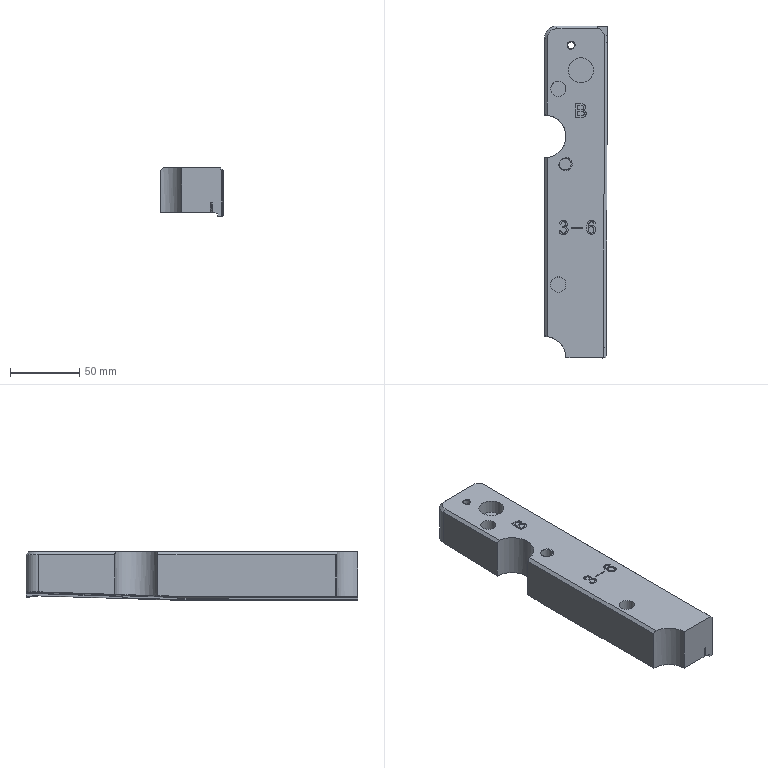NC program | NX | posted with a generic post | part box 45.476 x 239.737 x 35.001 mm
Lines 13412 to 14529 of 16758:
(CAVITY_MILL_2_COPY_COPY_COPY , TOOL : D8)
N26780 M6
N26782 G53
N26784 G17 G0 G90 X96.619 Y-3.563 S4500 M3
N26786 G43 Z60. H0
N26788 G94 G1 Z30.976 F4000.
N26790 Z30.776 F1380.
N26792 X91.019
N26794 Y-21.905 F2300.
N26796 X63.275
N26798 Y12.206
N26800 G3 X67.411 Y12.526 R72.418
N26802 G1 X82.944 Y15.381
N26804 X83.13 Y15.412
N26806 X86.93 Y15.616
N26808 G2 X91.019 Y15.688 R441.664
N26810 G1 Y-3.563
N26812 X85.819
N26814 Y-16.705
N26816 X68.475
N26818 Y7.435
N26820 X83.722 Y10.237
N26822 X85.819 Y10.349
N26824 Y-3.563
N26826 X80.619
N26828 Y-11.505
N26830 X73.675
N26832 Y3.103
N26834 X80.619 Y4.379
N26836 Y-3.563
N26838 X86.219
N26840 Z30.976
N26842 G0 Z60.
N26844 X96.619
N26846 G1 Z30.826 F4000.
N26848 Z30.626 F1380.
N26850 X91.019
N26852 Y-21.905 F2300.
N26854 X65.226
N26856 Y12.124
N26858 G3 X71.981 Y12.52 R70.87
N26860 G1 X87.545 Y15.381
N26862 X87.725 Y15.411
N26864 X91.019 Y15.583
N26866 Y-3.563
N26868 X85.819
N26870 Y-16.705
N26872 X70.426
N26874 Y7.154
N26876 G3 X72.533 Y7.35 R76.07
N26878 G1 X72.728 Y7.371
N26880 X85.819 Y9.776
N26882 Y-3.563
N26884 X80.619
N26886 Y-11.505
N26888 X75.626
N26890 Y2.616
N26892 X80.619 Y3.534
N26894 Y-3.563
N26896 X86.219
N26898 Z30.826
N26900 G0 Z60.
N26902 X96.619
N26904 G1 Z30.677 F4000.
N26906 Z30.477 F1380.
N26908 X91.019
N26910 Y-21.905 F2300.
N26912 X69.841
N26914 Y-13.95
N26916 X69.835 Y-13.743
N26918 X69.813 Y-13.538
N26920 G2 X69.841 Y-11.526 R10.118
N26922 G1 Y12.124
N26924 G3 X76.599 Y12.524 R71.863
N26926 G1 X91.019 Y15.174
N26928 Y-3.563
N26930 X85.819
N26932 Y-16.705
N26934 X75.041
N26936 Y-13.875
N26938 X75.027 Y-13.385
N26940 G2 X75.007 Y-12.116 R4.918
N26942 G1 X75.041 Y-11.822
N26944 Y7.157
N26946 G3 X77.151 Y7.353 R77.063
N26948 G1 X77.346 Y7.374
N26950 X85.819 Y8.931
N26952 Y-3.563
N26954 X80.619
N26956 Y-11.505
N26958 X80.241
N26960 Y2.619
N26962 X80.619 Y2.688
N26964 Y-3.563
N26966 X86.219
N26968 Z30.677
N26970 G0 Z60.
N26972 X96.619
N26974 G1 Z30.528 F4000.
N26976 Z30.328 F1380.
N26978 X91.019
N26980 Y-21.905 F2300.
N26982 X74.456
N26984 Y-20.642
N26986 X73.843 Y-18.475
N26988 G3 X71.487 Y-16.387 R16.517
N26990 G2 X71.487 Y-9.09 R4.8
N26992 G3 X74.456 Y-4.834 R7.409
N26994 G1 Y12.122
N26996 G3 X81.181 Y12.52 R74.277
N26998 G1 X91.019 Y14.328
N27000 Y-3.563
N27002 X85.819
N27004 Y-16.705
N27006 X78.733
N27008 G3 X77.647 Y-14.93 R5.2
N27010 X75.278 Y-12.739 R21.717
N27012 X79.493 Y-6.128 R12.609
N27014 G1 X79.656 Y-5.492
N27016 Y7.159
N27018 G3 X81.724 Y7.348 R79.477
N27020 G1 X81.924 Y7.369
N27022 X85.819 Y8.085
N27024 Y-3.563
N27026 X82.219 Y-9.282
N27028 Y-13.105
N27030 X80.815
N27032 G3 X80.361 Y-12.563 R8.8
N27034 X82.219 Y-9.282 R16.209
N27036 G1 X77.058 Y-7.109
N27038 Z30.528
N27040 G0 Z60.
N27042 X96.619 Y-3.563
N27044 G1 Z30.379 F4000.
N27046 Z30.179 F1380.
N27048 X91.019
N27050 Y-21.905 F2300.
N27052 X79.072
N27054 Y-21.737
N27056 X78.912 Y-21.048
N27058 G3 X74.547 Y-17.538 R4.537
N27060 G2 X73.96 Y-7.982 R4.8
N27062 G3 X79.032 Y-1.96 R6.196
N27064 G1 Y10.444
N27066 X79.072 Y11.241
N27068 Y12.122
N27070 X84.688 Y12.385
N27072 X85.787 Y12.521
N27074 X91.019 Y13.482
N27076 Y-3.563
N27078 X85.819
N27080 Y-16.705
N27082 X82.615
N27084 G3 X76.731 Y-12.598 R9.737
N27086 X84.232 Y-1.99 R11.396
N27088 G1 Y7.158
N27090 X85.129 Y7.2
N27092 X85.819 Y7.285
N27094 Y-3.563
N27096 X91.419
N27098 Z30.379
N27100 G0 Z60.
N27102 X96.619
N27104 G1 Z30.23 F4000.
N27106 Z30.03 F1380.
N27108 X91.019
N27110 Y-21.905 F2300.
N27112 X83.687
N27114 Y-20.591
N27116 X80.456 Y-16.221
N27118 X80.208 Y-16.188
N27120 G3 X77.104 Y-16.837 R4.742
N27122 G2 X73.96 Y-7.982 R-4.8
N27124 G3 X79.074 Y-1.875 R6.214
N27126 G1 Y10.544
N27128 G2 X79.429 Y11.192 R0.768
N27130 G3 X80.417 Y12.057 R4.366
N27132 G2 X80.618 Y12.081 R1.349
N27134 G3 X90.371 Y12.518 R96.02
N27136 G1 X91.019 Y12.637
N27138 Y-3.563
N27140 X85.819
N27142 Y-14.727
N27144 X84.637 Y-13.13
N27146 G3 X81.155 Y-11.068 R5.2
N27148 G1 X80.907 Y-11.035
N27150 G3 X79.776 Y-10.947 R9.942
N27152 G1 X74.95 Y-12.612
N27154 X79.776 Y-10.947
N27156 G3 X84.274 Y-1.879 R11.414
N27158 G1 Y6.926
N27160 G3 X85.819 Y6.984 R101.22
N27162 G1 Y-3.563
N27164 X91.419
N27166 Z30.23
N27168 G0 Z60.
N27170 X96.619
N27172 G1 Z30.081 F4000.
N27174 Z29.881 F1380.
N27176 X91.019
N27178 Y-21.905 F2300.
N27180 X88.303
N27182 Y-14.441
N27184 G3 X83.391 Y-10.449 R4.078
N27186 X79.726 Y-13.074 R5.582
N27188 X79.126 Y-14.354 R7.445
N27190 G2 X73.96 Y-7.982 R-4.8
N27192 G1 X74.771 Y-12.601
N27194 X73.96 Y-7.982
N27196 G3 X79.082 Y-1.874 R6.209
N27198 G1 Y10.538
N27200 G2 X79.438 Y11.19 R0.775
N27202 G3 X80.386 Y12.007 R4.443
N27204 G1 X88.702 Y12.127
N27206 G3 X91.019 Y12.201 R65.57
N27208 G1 Y-3.563
N27210 X85.819
N27212 Y-5.301
N27214 G3 X83.793 Y-5.173 R9.278
N27216 X84.282 Y-1.876 R11.409
N27218 G1 Y6.863
N27220 X85.819 Y6.885
N27222 Y-3.563
N27224 X91.419
N27226 Z30.081
N27228 G0 Z60.
N27230 X96.619
N27232 G1 Z29.932 F4000.
N27234 Z29.732 F1380.
N27236 X91.019
N27238 Y-10.908 F2300.
N27240 X90.885 Y-10.716
N27242 G3 X88.215 Y-10.089 R6.
N27244 G1 X85.018
N27246 G3 X79.191 Y-14.158 R6.217
N27248 G2 X73.96 Y-7.982 R-4.8
N27250 G1 X74.765 Y-12.604
N27252 X73.96 Y-7.982
N27254 G3 X79.09 Y-1.873 R6.209
N27256 G1 Y10.557
N27258 G2 X79.429 Y11.177 R0.735
N27260 G3 X80.387 Y11.996 R4.528
N27262 G1 X82.18
N27264 X88.919 Y12.058
N27266 X89.624
N27268 G3 X91.019 Y12.081 R144.478
N27270 G1 Y-3.563
N27272 X85.819
N27274 Y-4.889
N27276 X85.015
N27278 G3 X83.866 Y-4.948 R11.417
N27280 X84.29 Y-1.875 R11.409
N27282 G1 Y6.816
N27284 X85.819 Y6.829
N27286 Y-3.563
N27288 X91.419
N27290 Z29.932
N27292 G0 Z60.
N27294 X96.619
N27296 G1 Z29.783 F4000.
N27298 Z29.583 F1380.
N27300 X91.019
N27302 Y-10.082 F2300.
N27304 X85.02
N27306 G3 X79.191 Y-14.158 R6.214
N27308 G2 X73.96 Y-7.982 R-4.8
N27310 G1 X74.764 Y-12.605
N27312 X73.96 Y-7.982
N27314 G3 X79.097 Y-1.872 R6.209
N27316 G1 Y10.551
N27318 G2 X79.439 Y11.176 R0.743
N27320 G3 X80.395 Y11.995 R4.616
N27322 G1 X86.774
N27324 X87.156 Y11.997
N27326 X91.019 Y12.036
N27328 Y-3.563
N27330 X85.819
N27332 Y-4.882
N27334 X85.018
N27336 G3 X83.876 Y-4.94 R11.414
N27338 X84.297 Y-1.874 R11.409
N27340 G1 Y6.795
N27342 X85.819
N27344 Y-3.563
N27346 X91.419
N27348 Z29.783
N27350 G0 Z60.
N27352 X96.619
N27354 G1 Z29.634 F4000.
N27356 Z29.434 F1380.
N27358 X91.019
N27360 Y-10.074 F2300.
N27362 X85.023
N27364 G3 X79.191 Y-14.158 R6.216
N27366 G2 X73.96 Y-7.982 R-4.8
N27368 G1 X74.764 Y-12.605
N27370 X73.96 Y-7.982
N27372 G3 X79.105 Y-1.871 R6.208
N27374 G1 Y10.55
N27376 G2 X79.447 Y11.177 R0.744
N27378 G3 X80.404 Y11.994 R4.63
N27380 G1 X91.019
N27382 Y-3.563
N27384 X85.819
N27386 Y-4.874
N27388 X85.02
N27390 G3 X83.886 Y-4.931 R11.416
N27392 X84.305 Y-1.873 R11.408
N27394 G1 Y6.794
N27396 X85.819
N27398 Y-3.563
N27400 X91.419
N27402 Z29.634
N27404 G0 Z60.
N27406 X96.619
N27408 G1 Z29.484 F4000.
N27410 Z29.284 F1380.
N27412 X91.019
N27414 Y-10.066 F2300.
N27416 X85.025
N27418 G3 X79.191 Y-14.158 R6.216
N27420 G2 X73.96 Y-7.982 R-4.8
N27422 G1 X74.763 Y-12.606
N27424 X73.96 Y-7.982
N27426 G3 X79.113 Y-1.87 R6.208
N27428 G1 Y10.55
N27430 G2 X79.456 Y11.177 R0.746
N27432 G3 X80.413 Y11.993 R4.642
N27434 G1 X91.019
N27436 Y-3.563
N27438 X85.819
N27440 Y-4.866
N27442 X85.022
N27444 G3 X83.895 Y-4.923 R11.416
N27446 X84.313 Y-1.873 R11.408
N27448 G1 Y6.793
N27450 X85.819
N27452 Y-3.563
N27454 X91.419
N27456 Z29.484
N27458 G0 Z60.
N27460 X96.619
N27462 G1 Z29.335 F4000.
N27464 Z29.135 F1380.
N27466 X91.019
N27468 Y-10.058 F2300.
N27470 X85.028
N27472 G3 X79.191 Y-14.158 R6.211
N27474 G2 X73.96 Y-7.982 R-4.8
N27476 G1 X74.763 Y-12.606
N27478 X73.96 Y-7.982
N27480 G3 X79.121 Y-1.869 R6.208
N27482 G1 Y10.55
N27484 G2 X79.464 Y11.177 R0.745
N27486 G3 X80.421 Y11.991 R4.651
N27488 G1 X91.019
N27490 Y-3.563
N27492 X85.819
N27494 Y-4.858
N27496 X85.026
N27498 G3 X83.905 Y-4.914 R11.411
N27500 X84.321 Y-1.872 R11.408
N27502 G1 Y6.791
N27504 X85.819
N27506 Y-3.563
N27508 X91.419
N27510 Z29.335
N27512 G0 Z60.
N27514 X96.619
N27516 G1 Z29.186 F4000.
N27518 Z28.986 F1380.
N27520 X91.019
N27522 Y-10.05 F2300.
N27524 X85.03
N27526 G3 X79.191 Y-14.158 R6.211
N27528 G2 X73.96 Y-7.982 R-4.8
N27530 G1 X74.762 Y-12.606
N27532 X73.96 Y-7.982
N27534 G3 X79.129 Y-1.868 R6.208
N27536 G1 Y10.551
N27538 G2 X79.471 Y11.177 R0.742
N27540 G3 X80.43 Y11.99 R4.658
N27542 G1 X91.019
N27544 Y-3.563
N27546 X85.819
N27548 Y-4.85
N27550 X85.028
N27552 G3 X83.915 Y-4.905 R11.411
N27554 X84.329 Y-1.871 R11.408
N27556 G1 Y6.79
N27558 X85.819
N27560 Y-3.563
N27562 X91.419
N27564 Z29.186
N27566 G0 Z60.
N27568 X96.619
N27570 G1 Z29.037 F4000.
N27572 Z28.837 F1380.
N27574 X91.019
N27576 Y-10.043 F2300.
N27578 X85.033
N27580 G3 X79.191 Y-14.158 R6.211
N27582 G2 X73.96 Y-7.982 R-4.8
N27584 G1 X74.762 Y-12.607
N27586 X73.96 Y-7.982
N27588 G3 X79.137 Y-1.867 R6.207
N27590 G1 Y10.552
N27592 G2 X79.479 Y11.177 R0.74
N27594 G3 X80.438 Y11.989 R4.662
N27596 G1 X91.019
N27598 Y-3.563
N27600 X85.819
N27602 Y-4.843
N27604 X85.03
N27606 G3 X83.925 Y-4.897 R11.411
N27608 X84.337 Y-1.87 R11.407
N27610 G1 Y6.789
N27612 X85.819
N27614 Y-3.563
N27616 X91.419
N27618 Z29.037
N27620 G0 Z60.
N27622 X96.619
N27624 G1 Z28.888 F4000.
N27626 Z28.688 F1380.
N27628 X91.019
N27630 Y-10.035 F2300.
N27632 X85.035
N27634 G3 X79.191 Y-14.158 R6.211
N27636 G2 X73.96 Y-7.982 R-4.8
N27638 G1 X74.761 Y-12.607
N27640 X73.96 Y-7.982
N27642 G3 X79.144 Y-1.866 R6.207
N27644 G1 Y10.553
N27646 G2 X79.487 Y11.177 R0.739
N27648 G3 X80.447 Y11.987 R4.663
N27650 G1 X91.019
N27652 Y-3.563
N27654 X85.819
N27656 Y-4.835
N27658 X85.032
N27660 G3 X83.935 Y-4.888 R11.411
N27662 X84.344 Y-1.868 R11.407
N27664 G1 Y6.787
N27666 X85.819
N27668 Y-3.563
N27670 X91.419
N27672 Z28.888
N27674 G0 Z60.
N27676 X96.619
N27678 G1 Z28.739 F4000.
N27680 Z28.539 F1380.
N27682 X91.019
N27684 Y-10.027 F2300.
N27686 X85.037
N27688 G3 X79.191 Y-14.158 R6.211
N27690 G2 X73.96 Y-7.982 R-4.8
N27692 G1 X74.761 Y-12.608
N27694 X73.96 Y-7.982
N27696 G3 X79.152 Y-1.865 R6.207
N27698 G1 Y10.552
N27700 G2 X79.496 Y11.177 R0.741
N27702 G3 X80.455 Y11.986 R4.681
N27704 G1 X91.019
N27706 Y-3.563
N27708 X85.819
N27710 Y-4.827
N27712 X85.035
N27714 G3 X83.945 Y-4.88 R11.411
N27716 X84.352 Y-1.867 R11.407
N27718 G1 Y6.786
N27720 X85.819
N27722 Y-3.563
N27724 X91.419
N27726 Z28.739
N27728 G0 Z60.
N27730 X96.619
N27732 G1 Z28.59 F4000.
N27734 Z28.39 F1380.
N27736 X91.019
N27738 Y-10.019 F2300.
N27740 X85.04
N27742 G3 X79.191 Y-14.158 R6.212
N27744 G2 X73.96 Y-7.982 R-4.8
N27746 G1 X74.76 Y-12.608
N27748 X73.96 Y-7.982
N27750 G3 X79.16 Y-1.864 R6.207
N27752 G1 Y10.518
N27754 G2 X79.529 Y11.194 R0.804
N27756 G3 X80.464 Y11.985 R4.674
N27758 G1 X91.019
N27760 Y-3.563
N27762 X85.819
N27764 Y-4.819
N27766 X85.037
N27768 G3 X83.955 Y-4.871 R11.412
N27770 X84.36 Y-1.866 R11.407
N27772 G1 Y6.785
N27774 X85.819
N27776 Y-3.563
N27778 X91.419
N27780 Z28.59
N27782 G0 Z60.
N27784 X96.619
N27786 G1 Z28.441 F4000.
N27788 Z28.241 F1380.
N27790 X91.019
N27792 Y-10.011 F2300.
N27794 X85.042
N27796 G3 X79.191 Y-14.158 R6.212
N27798 G2 X73.96 Y-7.982 R-4.8
N27800 G1 X74.76 Y-12.609
N27802 X73.96 Y-7.982
N27804 G3 X79.168 Y-1.863 R6.206
N27806 G1 Y10.516
N27808 G2 X79.539 Y11.195 R0.807
N27810 G3 X80.472 Y11.983 R4.679
N27812 G1 X91.019
N27814 Y-3.563
N27816 X85.819
N27818 Y-4.811
N27820 X85.039
N27822 G3 X83.964 Y-4.863 R11.412
N27824 X84.368 Y-1.865 R11.406
N27826 G1 Y6.783
N27828 X85.819
N27830 Y-3.563
N27832 X91.419
N27834 Z28.441
N27836 G0 Z60.
N27838 X96.619
N27840 G1 Z28.292 F4000.
N27842 Z28.092 F1380.
N27844 X91.019
N27846 Y-10.003 F2300.
N27848 X85.045
N27850 G3 X79.191 Y-14.158 R6.212
N27852 G2 X73.96 Y-7.982 R-4.8
N27854 G1 X74.759 Y-12.609
N27856 X73.96 Y-7.982
N27858 G3 X79.176 Y-1.862 R6.206
N27860 G1 Y10.515
N27862 G2 X79.548 Y11.195 R0.808
N27864 G3 X80.481 Y11.982 R4.677
N27866 G1 X91.019
N27868 Y-3.563
N27870 X85.819
N27872 Y-4.803
N27874 X85.041
N27876 G3 X83.974 Y-4.854 R11.412
N27878 X84.376 Y-1.864 R11.406
N27880 G1 Y6.782
N27882 X85.819
N27884 Y-3.563
N27886 X91.419
N27888 Z28.292
N27890 G0 Z60.
N27892 X96.619
N27894 G1 Z28.143 F4000.
N27896 Z27.943 F1380.
N27898 X91.019
N27900 Y-9.996 F2300.
N27902 X85.047
N27904 G3 X79.191 Y-14.158 R6.212
N27906 G1 X74.759 Y-12.609
N27908 X79.191 Y-14.158
N27910 G2 X73.96 Y-7.982 R-4.8
N27912 G3 X79.183 Y-1.861 R6.205
N27914 G1 Y10.515
N27916 G2 X79.556 Y11.195 R0.807
N27918 G3 X80.489 Y11.981 R4.659
N27920 G1 X91.019
N27922 Y-3.563
N27924 X85.819
N27926 Y-4.796
N27928 X85.044
N27930 G3 X83.984 Y-4.846 R11.412
N27932 X84.383 Y-1.863 R11.405
N27934 G1 Y6.781
N27936 X85.819
N27938 Y-3.563
N27940 X91.419
N27942 Z28.143
N27944 G0 Z60.
N27946 X96.619
N27948 G1 Z27.993 F4000.
N27950 Z27.793 F1380.
N27952 X91.019
N27954 Y-9.988 F2300.
N27956 X85.05
N27958 G3 X79.191 Y-14.158 R6.207
N27960 G1 X74.758 Y-12.61
N27962 X79.191 Y-14.158
N27964 G2 X73.96 Y-7.982 R-4.8
N27966 G3 X79.191 Y-1.86 R6.205
N27968 G1 Y10.517
N27970 G2 X79.563 Y11.195 R0.803
N27972 G3 X80.497 Y11.98 R4.644
N27974 G1 X91.019
N27976 Y-3.563
N27978 X85.819
N27980 Y-4.788
N27982 X85.047
N27984 G3 X83.994 Y-4.837 R11.407
N27986 X84.391 Y-1.862 R11.405
N27988 G1 Y6.78
N27990 X85.819
N27992 Y-3.563
N27994 X91.419
N27996 Z27.993
N27998 G0 Z60.
N28000 X96.619
N28002 G1 Z27.844 F4000.
N28004 Z27.644 F1380.
N28006 X91.019
N28008 Y-9.98 F2300.
N28010 X85.052
N28012 G3 X79.191 Y-14.158 R6.207
N28014 G1 X74.758 Y-12.61
N28016 X79.191 Y-14.158
N28018 G2 X73.96 Y-7.982 R-4.8
N28020 G3 X79.199 Y-1.859 R6.205
N28022 G1 Y10.52
N28024 G2 X79.569 Y11.194 R0.798
N28026 G3 X80.505 Y11.978 R4.633
N28028 G1 X91.019
N28030 Y-3.563
N28032 X85.819
N28034 Y-4.78
N28036 X85.05
N28038 G3 X84.004 Y-4.829 R11.407
N28040 X84.399 Y-1.861 R11.405
N28042 G1 Y6.778
N28044 X85.819
N28046 Y-3.563
N28048 X91.419
N28050 Z27.844
N28052 G0 Z60.
N28054 X96.619
N28056 G1 Z27.695 F4000.
N28058 Z27.495 F1380.
N28060 X91.019
N28062 Y-9.972 F2300.
N28064 X85.054
N28066 G3 X79.191 Y-14.158 R6.207
N28068 G1 X74.757 Y-12.611
N28070 X79.191 Y-14.158
N28072 G2 X73.96 Y-7.982 R-4.8
N28074 G3 X79.207 Y-1.858 R6.204
N28076 G1 Y10.553
N28078 G2 X79.553 Y11.179 R0.738
N28080 G3 X80.515 Y11.977 R4.706
N28082 G1 X91.019
N28084 Y-3.563
N28086 X85.819
N28088 Y-4.772
N28090 X85.052
N28092 G3 X84.014 Y-4.82 R11.407
N28094 X84.407 Y-1.86 R11.404
N28096 G1 Y6.777
N28098 X85.819
N28100 Y-3.563
N28102 X91.419
N28104 Z27.695
N28106 G0 Z60.
N28108 X96.619
N28110 G1 Z27.546 F4000.
N28112 Z27.346 F1380.
N28114 X91.019
N28116 Y-9.964 F2300.
N28118 X85.057
N28120 G3 X79.191 Y-14.158 R6.207
N28122 G1 X74.757 Y-12.611
N28124 X79.191 Y-14.158
N28126 G2 X73.96 Y-7.982 R-4.8
N28128 G3 X79.215 Y-1.857 R6.204
N28130 G1 Y10.555
N28132 G2 X79.56 Y11.178 R0.735
N28134 G3 X80.523 Y11.976 R4.698
N28136 G1 X91.019
N28138 Y-3.563
N28140 X85.819
N28142 Y-4.764
N28144 X85.054
N28146 G3 X84.024 Y-4.812 R11.407
N28148 X84.415 Y-1.859 R11.404
N28150 G1 Y6.776
N28152 X85.819
N28154 Y-3.563
N28156 X91.419
N28158 Z27.546
N28160 G0 Z60.
N28162 X96.619
N28164 G1 Z27.397 F4000.
N28166 Z27.197 F1380.
N28168 X91.019
N28170 Y-9.957 F2300.
N28172 X85.059
N28174 G3 X79.191 Y-14.158 R6.207
N28176 G1 X74.756 Y-12.612
N28178 X79.191 Y-14.158
N28180 G2 X73.96 Y-7.982 R-4.8
N28182 G3 X79.223 Y-1.856 R6.203
N28184 G1 Y10.557
N28186 G2 X79.567 Y11.178 R0.731
N28188 G3 X80.531 Y11.974 R4.692
N28190 G1 X91.019
N28192 Y-3.563
N28194 X85.819
N28196 Y-4.757
N28198 X85.057
N28200 G3 X84.034 Y-4.803 R11.407
N28202 X84.423 Y-1.858 R11.403
N28204 G1 Y6.774
N28206 X85.819
N28208 Y-3.563
N28210 X91.419
N28212 Z27.397
N28214 G0 Z60.
N28216 X96.619
N28218 G1 Z27.248 F4000.
N28220 Z27.048 F1380.
N28222 X91.019
N28224 Y-9.949 F2300.
N28226 X85.062
N28228 G3 X79.191 Y-14.158 R6.212
N28230 G1 X74.756 Y-12.612
N28232 X79.191 Y-14.158
N28234 G2 X73.96 Y-7.982 R-4.8
N28236 G3 X79.23 Y-1.854 R6.203
N28238 G1 Y10.559
N28240 G2 X79.574 Y11.177 R0.727
N28242 G3 X80.54 Y11.973 R4.689
N28244 G1 X91.019
N28246 Y-3.563
N28248 X85.819
N28250 Y-4.749
N28252 X85.058
N28254 G3 X84.043 Y-4.795 R11.412
N28256 X84.43 Y-1.857 R11.403
N28258 G1 Y6.773
N28260 X85.819
N28262 Y-3.563
N28264 X91.419
N28266 Z27.248
N28268 G0 Z60.
N28270 X96.619
N28272 G1 Z27.099 F4000.
N28274 Z26.899 F1380.
N28276 X91.019
N28278 Y-9.941 F2300.
N28280 X85.064
N28282 G3 X79.191 Y-14.158 R6.212
N28284 G2 X74.049 Y-7.971 R-4.8
N28286 G1 X74.755 Y-12.614
N28288 X74.049 Y-7.971
N28290 G3 X79.238 Y-1.853 R6.208
N28292 G1 Y10.555
N28294 G2 X79.585 Y11.179 R0.734
N28296 G3 X80.548 Y11.972 R4.691
N28298 G1 X91.019
N28300 Y-3.563
N28302 X85.819
N28304 Y-4.741
N28306 X85.06
N28308 G3 X84.053 Y-4.787 R11.412
N28310 X84.438 Y-1.856 R11.408
N28312 G1 Y6.772
N28314 X85.819
N28316 Y-3.563
N28318 X91.419
N28320 Z27.099
N28322 G0 Z60.
N28324 X96.619
N28326 G1 Z26.95 F4000.
N28328 Z26.75 F1380.
N28330 X91.019
N28332 Y-9.933 F2300.
N28334 X85.067
N28336 G3 X79.191 Y-14.158 R6.212
N28338 G2 X74.049 Y-7.971 R-4.8
N28340 G1 X74.754 Y-12.614
N28342 X74.049 Y-7.971
N28344 G3 X79.246 Y-1.852 R6.208
N28346 G1 Y10.554
N28348 G2 X79.594 Y11.179 R0.735
N28350 G3 X80.556 Y11.97 R4.695
N28352 G1 X91.019
N28354 Y-3.563
N28356 X85.819
N28358 Y-4.733
N28360 X85.062
N28362 G3 X84.063 Y-4.778 R11.412
N28364 X84.446 Y-1.855 R11.408
N28366 G1 Y6.77
N28368 X85.819
N28370 Y-3.563
N28372 X91.419
N28374 Z26.95
N28376 G0 Z60.
N28378 X96.619
N28380 G1 Z26.801 F4000.
N28382 Z26.601 F1380.
N28384 X91.019
N28386 Y-9.925 F2300.
N28388 X85.069
N28390 G3 X79.191 Y-14.158 R6.21
N28392 G2 X74.049 Y-7.971 R-4.8
N28394 G1 X74.754 Y-12.614
N28396 X74.049 Y-7.971
N28398 G3 X79.254 Y-1.851 R6.207
N28400 G1 Y10.5
N28402 G2 X79.666 Y11.23 R0.853
N28404 G3 X80.566 Y11.969 R4.042
N28406 G1 X91.019
N28408 Y-3.563
N28410 X85.819
N28412 Y-4.725
N28414 X85.065
N28416 G3 X84.073 Y-4.77 R11.41
N28418 X84.454 Y-1.854 R11.407
N28420 G1 Y6.769
N28422 X85.819
N28424 Y-3.563
N28426 X91.419
N28428 Z26.801
N28430 G0 Z60.
N28432 X96.619
N28434 G1 Z26.651 F4000.
N28436 Z26.451 F1380.
N28438 X91.019
N28440 Y-9.917 F2300.
N28442 X85.071
N28444 G3 X79.191 Y-14.158 R6.21
N28446 G2 X74.049 Y-7.971 R-4.8
N28448 G1 X74.753 Y-12.615
N28450 X74.049 Y-7.971
N28452 G3 X79.262 Y-1.85 R6.206
N28454 G1 Y10.499
N28456 G2 X79.675 Y11.231 R0.854
N28458 G3 X80.574 Y11.968 R4.028
N28460 G1 X91.019
N28462 Y-3.563
N28464 X85.819
N28466 Y-4.717
N28468 X85.068
N28470 G3 X84.082 Y-4.761 R11.41
N28472 X84.462 Y-1.853 R11.406
N28474 G1 Y6.768
N28476 X85.819
N28478 Y-3.563
N28480 X91.419
N28482 Z26.651
N28484 G0 Z60.
N28486 X96.619
N28488 G1 Z26.502 F4000.
N28490 Z26.302 F1380.
N28492 X91.019
N28494 Y-9.91 F2300.
N28496 X85.074
N28498 G3 X79.191 Y-14.158 R6.213
N28500 G2 X74.049 Y-7.971 R-4.8
N28502 G1 X74.753 Y-12.615
N28504 X74.049 Y-7.971
N28506 G3 X79.269 Y-1.849 R6.205
N28508 G1 Y10.499
N28510 G2 X79.683 Y11.231 R0.853
N28512 G3 X80.582 Y11.967 R4.021
N28514 G1 X91.019
N28516 Y-3.563
N28518 X85.819
N28520 Y-4.71
N28522 X85.069
N28524 G3 X84.092 Y-4.753 R11.413
N28526 X84.469 Y-1.852 R11.405
N28528 G1 Y6.767
N28530 X85.819
N28532 Y-3.563
N28534 X91.419
N28536 Z26.502
N28538 G0 Z60.
N28540 X96.619
N28542 G1 Z26.353 F4000.
N28544 Z26.153 F1380.
N28546 X91.019
N28548 Y-9.902 F2300.
N28550 X85.076
N28552 G3 X79.212 Y-14.088 R6.217
N28554 G2 X74.049 Y-7.971 R-4.8
N28556 G1 X74.751 Y-12.616
N28558 X74.049 Y-7.971
N28560 G3 X79.277 Y-1.848 R6.205
N28562 G1 Y10.486
N28564 G2 X79.751 Y11.267 R0.861
N28566 G3 X80.591 Y11.965 R4.018
N28568 G1 X91.019
N28570 Y-3.563
N28572 X85.819
N28574 Y-4.702
N28576 X85.071
N28578 G3 X84.102 Y-4.745 R11.417
N28580 X84.477 Y-1.85 R11.405
N28582 G1 Y6.765
N28584 X85.819
N28586 Y-3.563
N28588 X91.419
N28590 Z26.353
N28592 G0 Z60.
N28594 X96.619
N28596 G1 Z26.204 F4000.
N28598 Z26.004 F1380.
N28600 X91.019
N28602 Y-9.894 F2300.
N28604 X85.079
N28606 G3 X79.212 Y-14.088 R6.217
N28608 G2 X74.049 Y-7.971 R-4.8
N28610 G1 X74.751 Y-12.616
N28612 X74.049 Y-7.971
N28614 G3 X79.285 Y-1.847 R6.204
N28616 G1 Y10.486
N28618 G2 X79.751 Y11.262 R0.855
N28620 G3 X80.6 Y11.964 R4.091
N28622 G1 X91.019
N28624 Y-3.563
N28626 X85.819
N28628 Y-4.694
N28630 X85.074
N28632 G3 X84.112 Y-4.736 R11.417
N28634 X84.485 Y-1.849 R11.404
N28636 G1 Y6.764
N28638 X85.819
N28640 Y-3.563
N28642 X91.419
N28644 Z26.204
N28646 G0 Z60.
N28648 X96.619
N28650 G1 Z26.055 F4000.
N28652 Z25.855 F1380.
N28654 X91.019
N28656 Y-9.886 F2300.
N28658 X85.081
N28660 G3 X79.212 Y-14.088 R6.221
N28662 G2 X74.049 Y-7.971 R-4.8
N28664 G1 X74.75 Y-12.617
N28666 X74.049 Y-7.971
N28668 G3 X79.293 Y-1.846 R6.203
N28670 G1 Y10.486
N28672 G2 X79.751 Y11.257 R0.847
N28674 G3 X80.608 Y11.963 R4.1
N28676 G1 X91.019
N28678 Y-3.563
N28680 X85.819
N28682 Y-4.686
N28684 X85.075
N28686 G3 X84.122 Y-4.728 R11.421
N28688 X84.493 Y-1.848 R11.403
N28690 G1 Y6.763
N28692 X85.819
N28694 Y-3.563
N28696 X91.419
N28698 Z26.055
N28700 G0 Z60.
N28702 X96.619
N28704 G1 Z25.906 F4000.
N28706 Z25.706 F1380.
N28708 X91.019
N28710 Y-9.878 F2300.
N28712 X85.084
N28714 G3 X79.212 Y-14.088 R6.221
N28716 G2 X74.049 Y-7.971 R-4.8
N28718 G1 X74.75 Y-12.617
N28720 X74.049 Y-7.971
N28722 G3 X79.301 Y-1.845 R6.202
N28724 G1 Y10.486
N28726 G2 X79.751 Y11.251 R0.838
N28728 G3 X80.617 Y11.961 R4.108
N28730 G1 X91.019
N28732 Y-3.563
N28734 X85.819
N28736 Y-4.678
N28738 X85.077
N28740 G3 X84.132 Y-4.719 R11.421
N28742 X84.501 Y-1.847 R11.402
N28744 G1 Y6.761
N28746 X85.819
N28748 Y-3.563
N28750 X91.419
N28752 Z25.906
N28754 G0 Z60.
N28756 X96.619
N28758 G1 Z25.757 F4000.
N28760 Z25.557 F1380.
N28762 X91.019
N28764 Y-9.871 F2300.
N28766 X85.086
N28768 G3 X79.212 Y-14.088 R6.216
N28770 G2 X74.049 Y-7.971 R-4.8
N28772 G1 X74.749 Y-12.618
N28774 X74.049 Y-7.971
N28776 G3 X79.308 Y-1.844 R6.201
N28778 G1 Y10.486
N28780 G2 X79.751 Y11.246 R0.831
N28782 G3 X80.625 Y11.96 R4.121
N28784 G1 X91.019
N28786 Y-3.563
N28788 X85.819
N28790 Y-4.671
N28792 X85.081
N28794 G3 X84.141 Y-4.711 R11.416
N28796 X84.508 Y-1.847 R11.401
N28798 G1 Y6.76
N28800 X85.819
N28802 Y-3.563
N28804 X91.419
N28806 Z25.757
N28808 G0 Z60.
N28810 X96.619
N28812 G1 Z25.608 F4000.
N28814 Z25.408 F1380.
N28816 X91.019
N28818 Y-9.863 F2300.
N28820 X85.089
N28822 G3 X79.224 Y-14.047 R6.222
N28824 G2 X74.049 Y-7.971 R-4.8
N28826 G1 X74.748 Y-12.618
N28828 X74.049 Y-7.971
N28830 G3 X79.316 Y-1.843 R6.201
N28832 G1 Y10.486
N28834 G2 X79.751 Y11.241 R0.823
N28836 G3 X80.635 Y11.959 R4.186
N28838 G1 X91.019
N28840 Y-3.563
N28842 X85.819
N28844 Y-4.663
N28846 X85.082
N28848 G3 X84.151 Y-4.703 R11.422
N28850 X84.516 Y-1.845 R11.401
N28852 G1 Y6.759
N28854 X85.819
N28856 Y-3.563
N28858 X91.419
N28860 Z25.608
N28862 G0 Z60.
N28864 X96.619
N28866 G1 Z25.459 F4000.
N28868 Z25.259 F1380.
N28870 X91.019
N28872 Y-9.855 F2300.
N28874 X85.091
N28876 G3 X79.224 Y-14.047 R6.222
N28878 G2 X74.049 Y-7.971 R-4.8
N28880 G1 X74.748 Y-12.619
N28882 X74.049 Y-7.971
N28884 G3 X79.324 Y-1.842 R6.201
N28886 G1 Y10.486
N28888 G2 X79.751 Y11.236 R0.815
N28890 G3 X80.643 Y11.957 R4.201
N28892 G1 X91.019
N28894 Y-3.563
N28896 X85.819
N28898 Y-4.655
N28900 X85.085
N28902 G3 X84.161 Y-4.694 R11.422
N28904 X84.524 Y-1.844 R11.401
N28906 G1 Y6.757
N28908 X85.819
N28910 Y-3.563
N28912 X91.419
N28914 Z25.459
N28916 G0 Z60.
N28918 X96.619
N28920 G1 Z25.31 F4000.
N28922 Z25.11 F1380.
N28924 X91.019
N28926 Y-9.847 F2300.
N28928 X85.093
N28930 G3 X79.224 Y-14.047 R6.222
N28932 G2 X74.049 Y-7.971 R-4.8
N28934 G1 X74.747 Y-12.619
N28936 X74.049 Y-7.971
N28938 G3 X79.332 Y-1.841 R6.2
N28940 G1 Y10.486
N28942 G2 X79.751 Y11.23 R0.809
N28944 G3 X80.651 Y11.956 R4.214
N28946 G1 X91.019
N28948 Y-3.563
N28950 X85.819
N28952 Y-4.647
N28954 X85.087
N28956 G3 X84.171 Y-4.686 R11.422
N28958 X84.532 Y-1.843 R11.4
N28960 G1 Y6.756
N28962 X85.819
N28964 Y-3.563
N28966 X91.419
N28968 Z25.31
N28970 G0 Z60.
N28972 X96.619
N28974 G1 Z25.16 F4000.
N28976 Z24.96 F1380.
N28978 X91.019
N28980 Y-9.839 F2300.
N28982 X85.096
N28984 G3 X79.224 Y-14.047 R6.221
N28986 G2 X74.049 Y-7.971 R-4.8
N28988 G1 X74.747 Y-12.619
N28990 X74.049 Y-7.971
N28992 G3 X79.34 Y-1.84 R6.2
N28994 G1 Y10.486
N28996 G2 X79.751 Y11.225 R0.821
N28998 G3 X80.659 Y11.955 R4.231
N29000 G1 X91.019
N29002 Y-3.563
N29004 X85.819
N29006 Y-4.639
N29008 X85.09